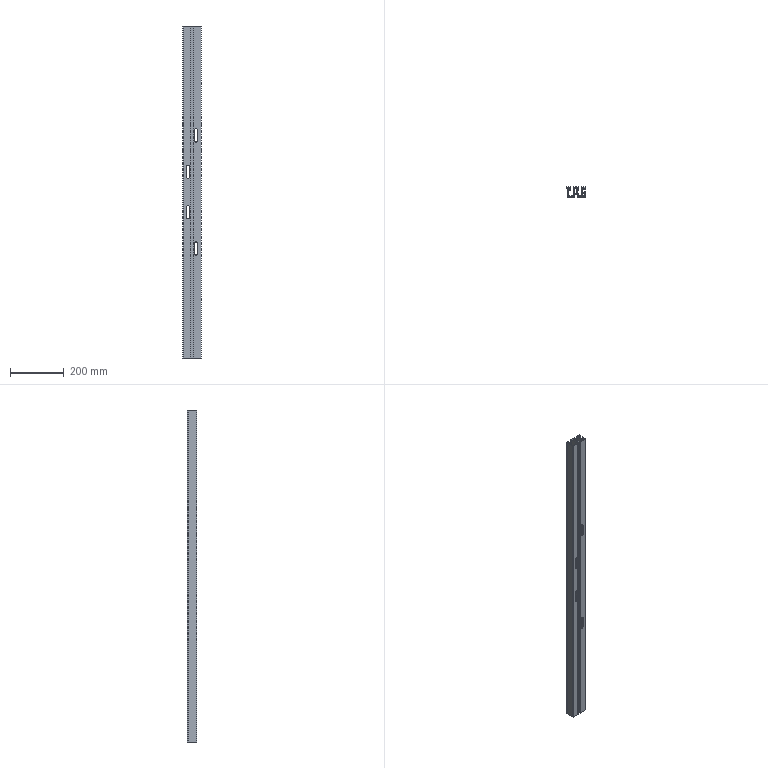Part | 1 solid | 95 faces | box 70 x 35 x 1230 mm | volume 881214 mm3 | plane 66 | cylinder 29 | commonest cylinder face diameters 9 x12 2 x8 5 x4 3 x3 1 x1 4 x1